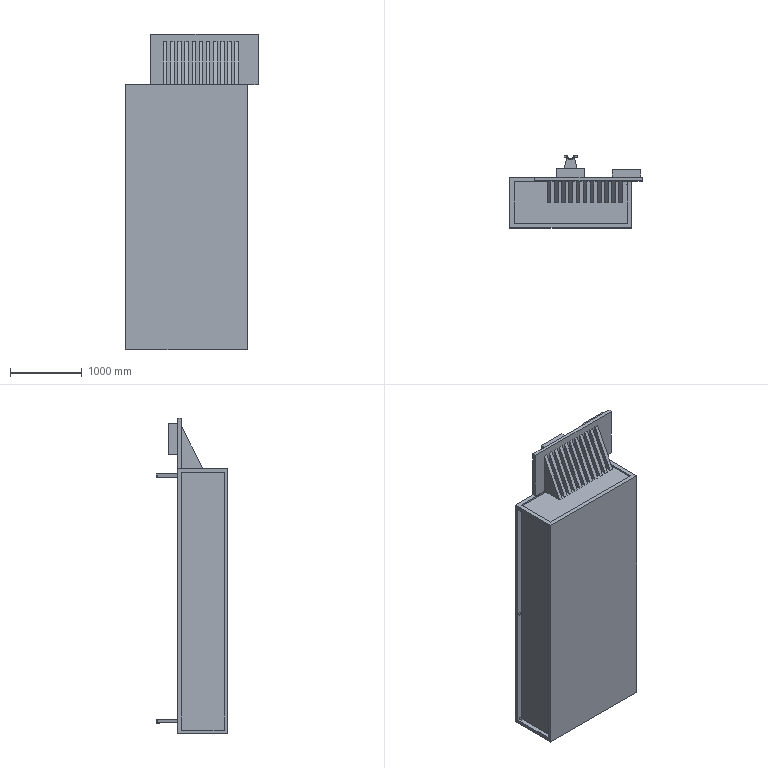Part | SolidWorks | features ICE 35, LPattern 2, Extrusion 1 | 1 solid | 166 faces | box 1850 x 1000 x 4400 mm | volume 1049313623 mm3 | plane 130 | cylinder 36 | commonest cylinder face diameters 12 x16 40 x12 50 x2 90 x2 105 x2 75.1 x1